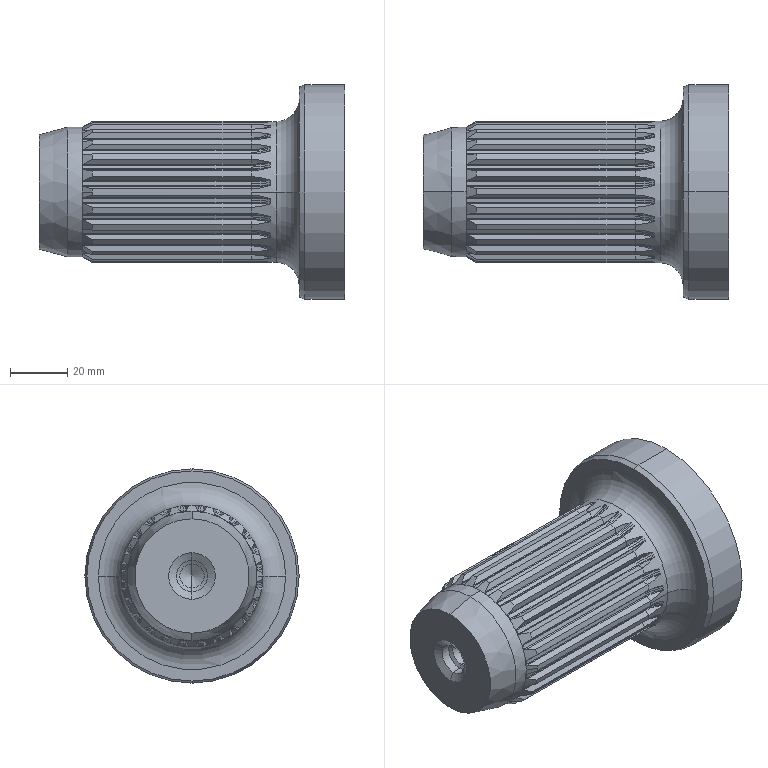Part | SolidWorks | features BaseBody 1 | 1 solid | 316 faces | box 107 x 75 x 75 mm | volume 230700 mm3 | spline 241 | torus 50 | cone 12 | cylinder 10 | plane 3 | commonest cylinder face diameters 8.5 x2 11 x2 45.4 x2 49.6 x2 75 x2